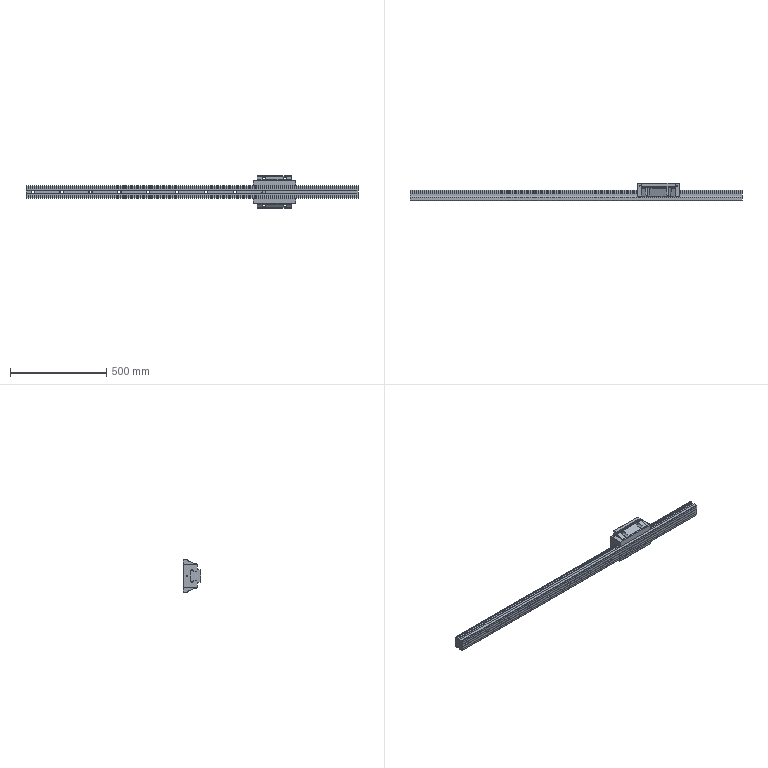Part | SolidWorks | 2 solids | 284 faces | box 1725 x 90 x 170 mm | volume 6825649 mm3 | plane 152 | cylinder 104 | cone 28 | commonest cylinder face diameters 1 x20 18 x18 26 x18 6 x12 5.2 x8 9.8 x8